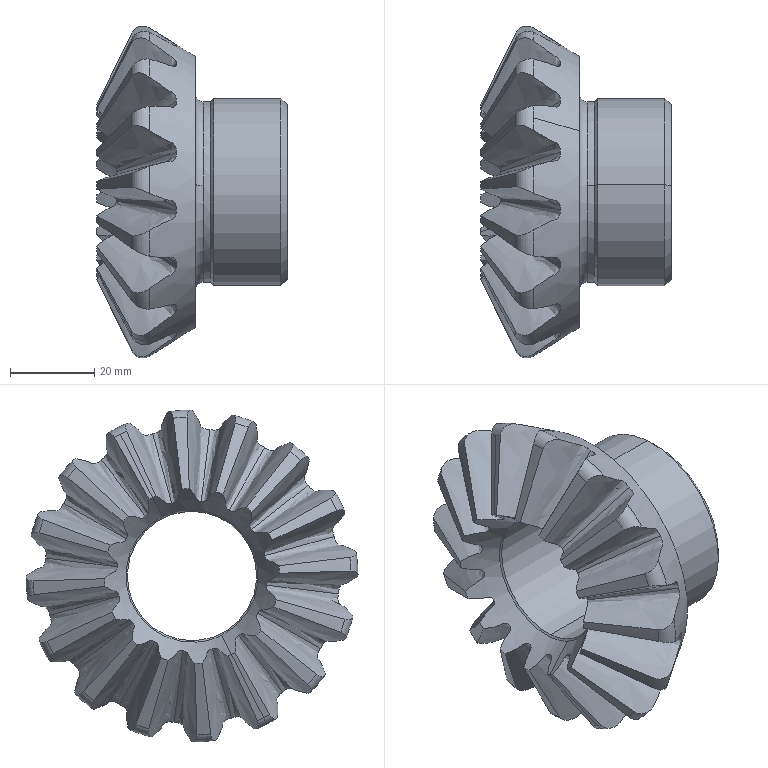Part | NX | features BREP 1 | 1 solid | 90 faces | box 45.113 x 78.686 x 78.686 mm | volume 67426 mm3 | spline 32 | cone 30 | torus 20 | cylinder 6 | plane 2 | commonest cylinder face diameters 30.66 x2 42.88 x2 44.4 x2